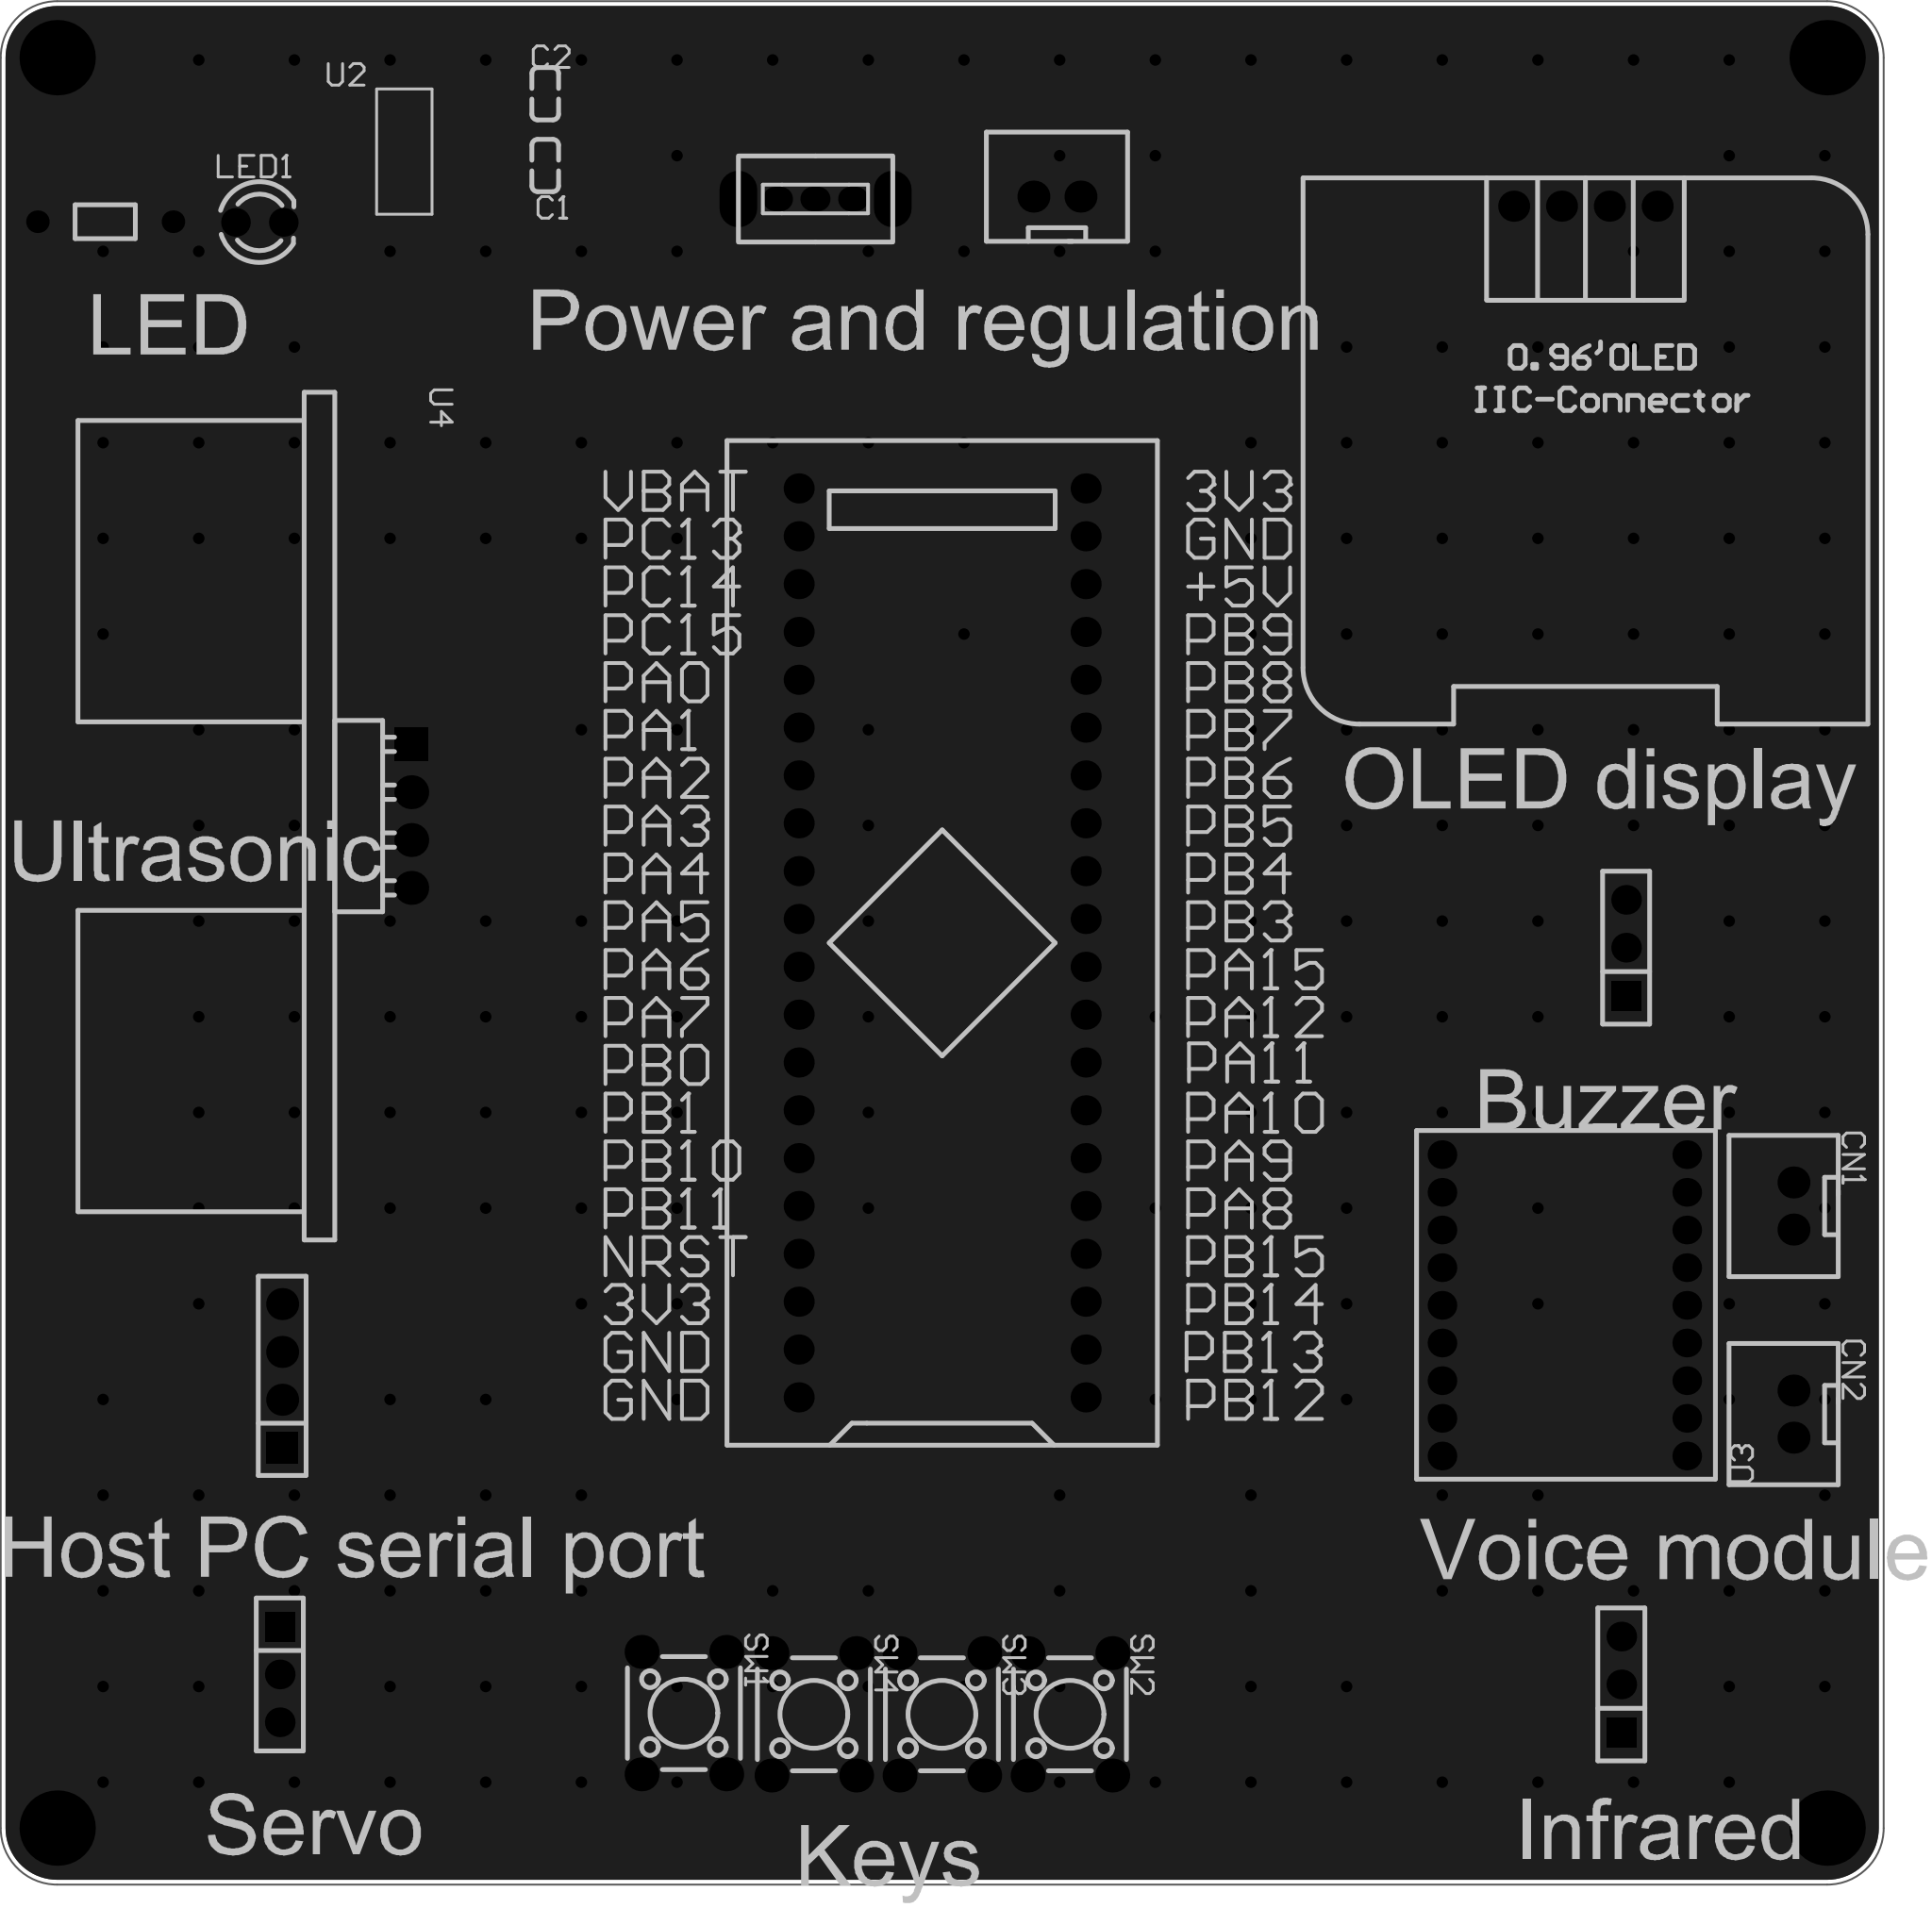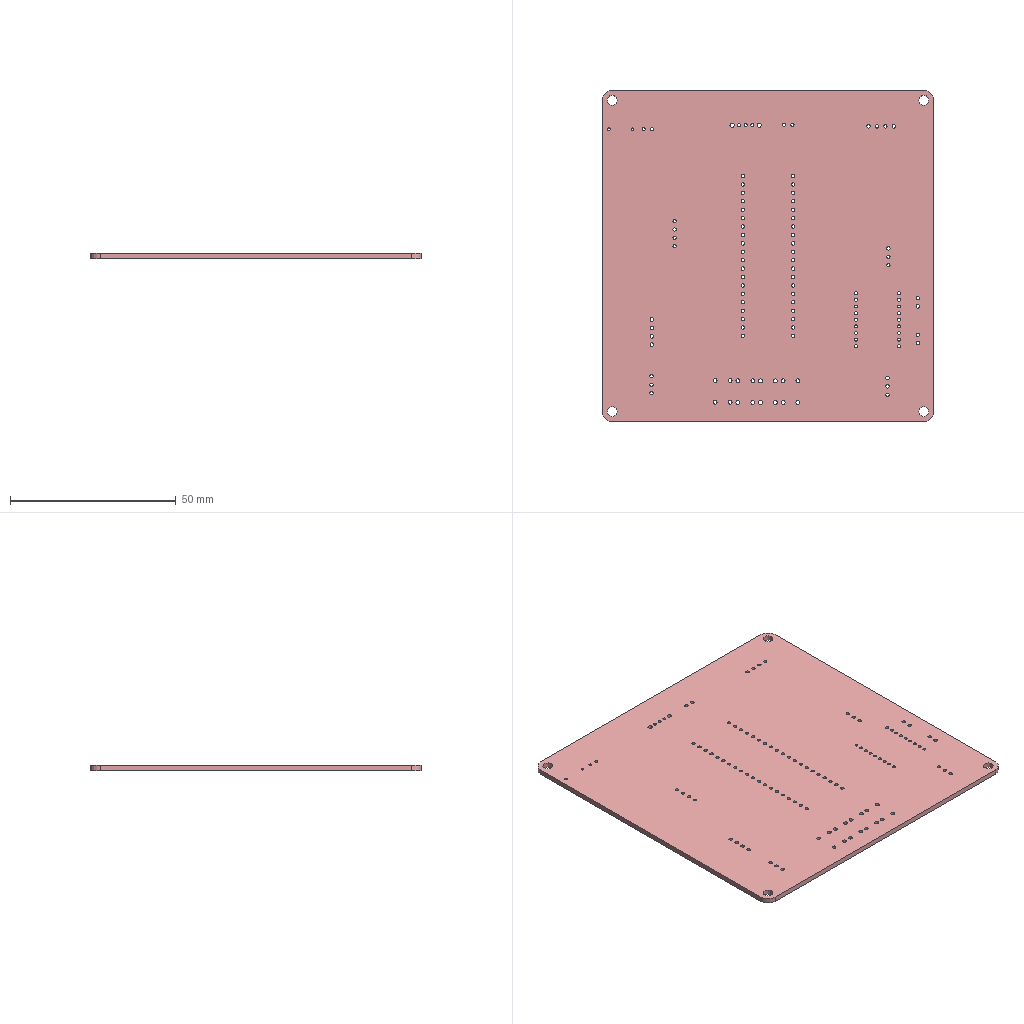Circuit board layout | Altium Designer | box 100 x 100 x 1.6 mm
Layer stack:
# Altium Designer layer stack of  (unit mm; dielectric type: 0 none, 1 core, 2 prepreg, 3 surface material)
index,name,kind,layer,copper_thickness_mm,dielectric_type,dielectric_thickness_mm,dielectric_material,dielectric_constant
0,Top Paste Mask Layer,other,,,,,,
1,Top Silkscreen Layer,other,,,,,,
2,Top Solder Mask Layer,dielectric,,,3,0.01,,3.3
3,Top Layer,copper,Top Layer,0.035,,,,
4,Dielectric1,dielectric,,,3,1.51,FR4,4.5
5,Bottom Layer,copper,Bottom Layer,0.035,,,,
6,Bottom Solder Mask Layer,dielectric,,,3,0.01,,3.3
7,Bottom Silkscreen Layer,other,,,,,,
8,Bottom Paste Mask Layer,other,,,,,,
# drill layer pairs: low layer,high layer
drill_pair,Top Layer,Bottom Layer
Part placement:
Designator,Comment,Layer,Footprint,Center-X(mm),Center-Y(mm),Rotation
U1,STM32F103C8T6-Card,TopLayer,CONN-TH_L53.3-W22.9_STM32F103C8T6-CARD,141.351,130.937,90
OLED1,,TopLayer,0.96OLED_4P,175.514,170.053,0
SW1,,TopLayer,SW-TH_4P-L6.0-W6.0-P4.50-LS6.5,127.635,90.043,270
SW2,,TopLayer,SW-TH_4P-L6.0-W6.0-P4.50-LS6.5,148.136,89.979,270
SW3,,TopLayer,SW-TH_4P-L6.0-W6.0-P4.50-LS6.5,141.337,89.979,270
SW4,,TopLayer,SW-TH_4P-L6.0-W6.0-P4.50-LS6.5,134.537,89.979,270
H12,,TopLayer,HDR-TH_3P-P2.54-V-F,106.172,92.095,270
CN4,XH2.54*2P_through-hole,TopLayer,CONN-TH_2P-P2.50-XH2.54-2P,147.447,170.561,180
SW5,,TopLayer,拨动开关,134.628,170.434,0
H1,,TopLayer,HDR-TH_3P-P2.54-V-F,177.673,130.683,90
H2,,TopLayer,HDR-TH_4P-P2.54-V-F,106.299,107.95,90
H3,,TopLayer,HDR-TH_3P-P2.54-V-F,177.419,91.567,90
C1,100nF,TopLayer,C0603,120.269,172.212,90
C2,100nF,TopLayer,C0603,120.269,176.022,270
CN1,XH2.54*2P_through-hole,TopLayer,CONN-TH_2P-P2.50-XH2.54-2P,186.563,116.967,270
CN2,XH2.54*2P_through-hole,TopLayer,CONN-TH_2P-P2.50-XH2.54-2P,186.563,105.918,270
R1,220Ω,TopLayer,Res_1/8W,96.901,169.228,180
LED1,,TopLayer,LED_TH-3mm,105.091,169.193,0
U2,AMS1117-3.3,TopLayer,SOT-223-3_L6.5-W3.4-P2.30-LS7.0-BR,112.886,172.951,0
U3,CON2.0MM-PAD-18,TopLayer,CONN-TH_18P-P2.00_C9900078766,174.395,111.693,90
U4,HC-SR04,TopLayer,TH_HC-SR04V,113.157,137.668,270
Pad and via stacks:
# Altium Designer via and pad stacks of  (unit mm). Each distinct definition once, with the count of objects using it.
# via: kind,start_layer,end_layer,hole_mm,diameter_mm,mode(0 simple;1 top-mid-bottom;2 full stack),diameter_per_layer,count,example_net
# pad: kind,layer,hole_mm,hole_type(0 round;1 square;2 slot),plating,top_size,top_shape(1 round;2 rect;3 octagon;9 rounded rect),mid_size,bottom_size,mode,footprint,size_per_layer,count,example
pad,Multi-Layer,3,0,plated,4x4,1,4x4,4x4,0,,,4,1
pad,Multi-Layer,1,0,plated,1.6x1.6,1,1.6x1.6,1.6x1.6,0,CONN-TH_L53.3-W22.9_STM32F103C8T6-CARD,,40,U1.1
pad,Multi-Layer,1,0,plated,1.65x1.65,1,1.65x1.65,1.65x1.65,0,0.96OLED_4P,,4,OLED1.4
pad,Multi-Layer,1.2,0,plated,1.8x1.8,1,1.8x1.8,1.8x1.8,0,SW-TH_4P-L6.0-W6.0-P4.50-LS6.5,,16,SW1.1
pad,Multi-Layer,1.02,0,plated,1.575x1.575,1,1.575x1.575,1.575x1.575,0,HDR-TH_3P-P2.54-V-F,,6,H12.3
pad,Multi-Layer,1.02,0,plated,1.575x1.575,2,1.575x1.575,1.575x1.575,0,HDR-TH_3P-P2.54-V-F,,3,H12.1
pad,Multi-Layer,1.05,0,plated,1.7x1.7,1,1.7x1.7,1.7x1.7,0,CONN-TH_2P-P2.50-XH2.54-2P,,6,CN4.2
pad,Multi-Layer,0.8992,0,plated,1.6x1.3,1,1.6x1.3,1.6x1.3,0,\u00B2\u00A6\u00B6\u00AF\u00BF\u00AA\u00B9\u00D8,,3,SW5.1
pad,Multi-Layer,1.3,0,plated,3x1.999,1,3x1.999,3x1.999,0,\u00B2\u00A6\u00B6\u00AF\u00BF\u00AA\u00B9\u00D8,,2,SW5.4
pad,Multi-Layer,1.1,0,plated,1.7x1.7,2,1.7x1.7,1.7x1.7,0,HDR-TH_4P-P2.54-V-F,,1,H2.1
pad,Multi-Layer,1.1,0,plated,1.7x1.7,1,1.7x1.7,1.7x1.7,0,HDR-TH_4P-P2.54-V-F,,3,H2.2
pad,Multi-Layer,0.8001,0,plated,1.199x1.199,1,1.199x1.199,1.199x1.199,0,Res_1/8W,,2,R1.1
pad,Multi-Layer,0.9144,0,plated,1.524x1.524,1,1.524x1.524,1.524x1.524,0,LED_TH-3mm,,2,LED1.1
pad,Multi-Layer,0.9,0,plated,1.524x1.524,1,1.524x1.524,1.524x1.524,0,CONN-TH_18P-P2.00_C9900078766,,18,U3.1
pad,Multi-Layer,1.001,0,plated,1.8x1.8,1,1.8x1.8,1.8x1.8,0,TH_HC-SR04V,,3,U4.4
pad,Multi-Layer,1.001,0,plated,1.8x1.8,2,1.8x1.8,1.8x1.8,0,TH_HC-SR04V,,1,U4.1
pad,Top Layer,0,0,plated,0.8x0.9,2,0.8x0.9,0.8x0.9,0,C0603,,4,C1.2
pad,Top Layer,0,0,plated,2.5x1.1,2,2.5x1.1,2.5x1.1,0,SOT-223-3_L6.5-W3.4-P2.30-LS7.0-BR,,3,U2.1
pad,Top Layer,0,0,plated,2.34x3.6,2,2.34x3.6,2.34x3.6,0,SOT-223-3_L6.5-W3.4-P2.30-LS7.0-BR,,1,U2.4
via,Top Layer,Bottom Layer,0.3048,0.61,0,,230,GND
Copper pours:
name,layer,net,type(0 solid;1 hatched;2 none)
Bottom Layer-GND,Bottom Layer,GND,0
Top Layer-GND,Top Layer,GND,0